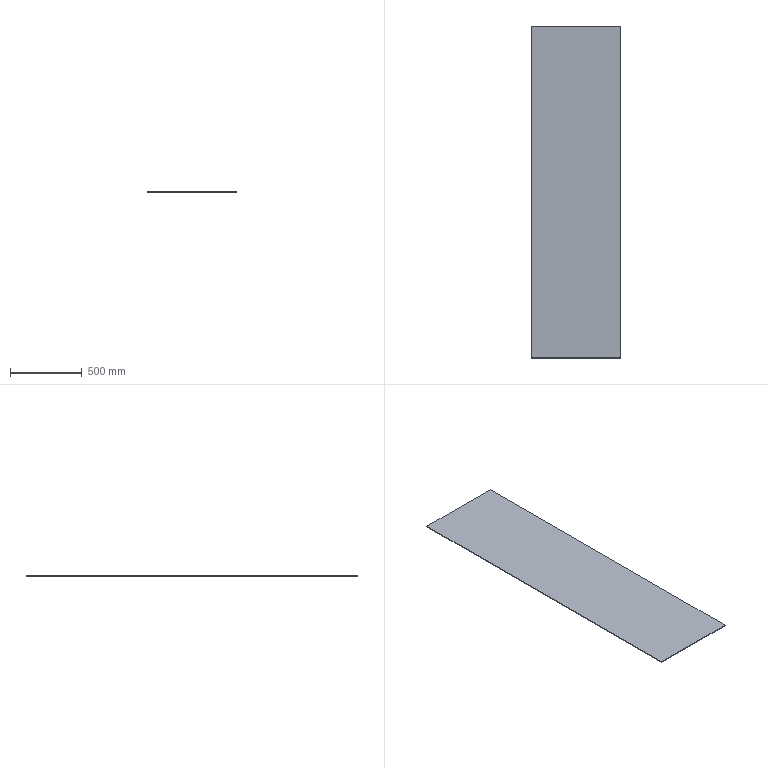Part | SolidWorks | features Extrusion 1, HoleWzd 1 | 1 solid | 6 faces | box 624 x 2310 x 5 mm | volume 7207200 mm3 | plane 6
STEP:
#1=CARTESIAN_POINT('',(312.,-1155.,0.));
#2=VERTEX_POINT('',#1);
#3=CARTESIAN_POINT('',(312.,1155.,0.));
#4=VERTEX_POINT('',#3);
#5=CARTESIAN_POINT('',(312.,1155.,0.));
#6=DIRECTION('',(0.,1.,0.));
#7=VECTOR('',#6,1000.);
#8=LINE('',#5,#7);
#9=EDGE_CURVE('',#2,#4,#8,.T.);
#10=ORIENTED_EDGE('',*,*,#9,.T.);
#11=CARTESIAN_POINT('',(312.,1155.,5.));
#12=VERTEX_POINT('',#11);
#13=CARTESIAN_POINT('',(312.,1155.,5.));
#14=DIRECTION('',(0.,0.,-1.));
#15=VECTOR('',#14,1000.);
#16=LINE('',#13,#15);
#17=EDGE_CURVE('',#12,#4,#16,.T.);
#18=ORIENTED_EDGE('',*,*,#17,.F.);
#19=CARTESIAN_POINT('',(312.,-1155.,5.));
#20=VERTEX_POINT('',#19);
#21=CARTESIAN_POINT('',(312.,1155.,5.));
#22=DIRECTION('',(0.,1.,0.));
#23=VECTOR('',#22,1000.);
#24=LINE('',#21,#23);
#25=EDGE_CURVE('',#20,#12,#24,.T.);
#26=ORIENTED_EDGE('',*,*,#25,.F.);
#27=CARTESIAN_POINT('',(312.,-1155.,5.));
#28=DIRECTION('',(0.,0.,-1.));
#29=VECTOR('',#28,1000.);
#30=LINE('',#27,#29);
#31=EDGE_CURVE('',#20,#2,#30,.T.);
#32=ORIENTED_EDGE('',*,*,#31,.T.);
#33=EDGE_LOOP('',(#10,#18,#26,#32));
#34=FACE_OUTER_BOUND('',#33,.T.);
#35=CARTESIAN_POINT('',(312.,1155.,5.));
#36=DIRECTION('',(-1.,0.,0.));
#37=DIRECTION('',(0.,-1.,0.));
#38=AXIS2_PLACEMENT_3D('',#35,#36,#37);
#39=PLANE('',#38);
#40=ADVANCED_FACE('',(#34),#39,.F.);
#41=CARTESIAN_POINT('',(-312.,1155.,0.));
#42=VERTEX_POINT('',#41);
#43=CARTESIAN_POINT('',(-312.,1155.,0.));
#44=DIRECTION('',(-1.,0.,0.));
#45=VECTOR('',#44,1000.);
#46=LINE('',#43,#45);
#47=EDGE_CURVE('',#4,#42,#46,.T.);
#48=ORIENTED_EDGE('',*,*,#47,.T.);
#49=CARTESIAN_POINT('',(-312.,1155.,5.));
#50=VERTEX_POINT('',#49);
#51=CARTESIAN_POINT('',(-312.,1155.,5.));
#52=DIRECTION('',(0.,0.,-1.));
#53=VECTOR('',#52,1000.);
#54=LINE('',#51,#53);
#55=EDGE_CURVE('',#50,#42,#54,.T.);
#56=ORIENTED_EDGE('',*,*,#55,.F.);
#57=CARTESIAN_POINT('',(-312.,1155.,5.));
#58=DIRECTION('',(-1.,0.,0.));
#59=VECTOR('',#58,1000.);
#60=LINE('',#57,#59);
#61=EDGE_CURVE('',#12,#50,#60,.T.);
#62=ORIENTED_EDGE('',*,*,#61,.F.);
#63=ORIENTED_EDGE('',*,*,#17,.T.);
#64=EDGE_LOOP('',(#48,#56,#62,#63));
#65=FACE_OUTER_BOUND('',#64,.T.);
#66=CARTESIAN_POINT('',(-312.,1155.,5.));
#67=DIRECTION('',(0.,-1.,0.));
#68=DIRECTION('',(0.,0.,-1.));
#69=AXIS2_PLACEMENT_3D('',#66,#67,#68);
#70=PLANE('',#69);
#71=ADVANCED_FACE('',(#65),#70,.F.);
#72=CARTESIAN_POINT('',(-312.,-1155.,0.));
#73=VERTEX_POINT('',#72);
#74=CARTESIAN_POINT('',(-312.,1155.,0.));
#75=DIRECTION('',(0.,-1.,0.));
#76=VECTOR('',#75,1000.);
#77=LINE('',#74,#76);
#78=EDGE_CURVE('',#42,#73,#77,.T.);
#79=ORIENTED_EDGE('',*,*,#78,.T.);
#80=CARTESIAN_POINT('',(-312.,-1155.,5.));
#81=VERTEX_POINT('',#80);
#82=CARTESIAN_POINT('',(-312.,-1155.,5.));
#83=DIRECTION('',(0.,0.,-1.));
#84=VECTOR('',#83,1000.);
#85=LINE('',#82,#84);
#86=EDGE_CURVE('',#81,#73,#85,.T.);
#87=ORIENTED_EDGE('',*,*,#86,.F.);
#88=CARTESIAN_POINT('',(-312.,1155.,5.));
#89=DIRECTION('',(0.,-1.,0.));
#90=VECTOR('',#89,1000.);
#91=LINE('',#88,#90);
#92=EDGE_CURVE('',#50,#81,#91,.T.);
#93=ORIENTED_EDGE('',*,*,#92,.F.);
#94=ORIENTED_EDGE('',*,*,#55,.T.);
#95=EDGE_LOOP('',(#79,#87,#93,#94));
#96=FACE_OUTER_BOUND('',#95,.T.);
#97=CARTESIAN_POINT('',(-312.,1155.,5.));
#98=DIRECTION('',(1.,0.,0.));
#99=DIRECTION('',(0.,1.,0.));
#100=AXIS2_PLACEMENT_3D('',#97,#98,#99);
#101=PLANE('',#100);
#102=ADVANCED_FACE('',(#96),#101,.F.);
#103=CARTESIAN_POINT('',(-312.,-1155.,0.));
#104=DIRECTION('',(1.,0.,0.));
#105=VECTOR('',#104,1000.);
#106=LINE('',#103,#105);
#107=EDGE_CURVE('',#73,#2,#106,.T.);
#108=ORIENTED_EDGE('',*,*,#107,.T.);
#109=ORIENTED_EDGE('',*,*,#31,.F.);
#110=CARTESIAN_POINT('',(-312.,-1155.,5.));
#111=DIRECTION('',(1.,0.,0.));
#112=VECTOR('',#111,1000.);
#113=LINE('',#110,#112);
#114=EDGE_CURVE('',#81,#20,#113,.T.);
#115=ORIENTED_EDGE('',*,*,#114,.F.);
#116=ORIENTED_EDGE('',*,*,#86,.T.);
#117=EDGE_LOOP('',(#108,#109,#115,#116));
#118=FACE_OUTER_BOUND('',#117,.T.);
#119=CARTESIAN_POINT('',(-312.,-1155.,5.));
#120=DIRECTION('',(0.,1.,0.));
#121=DIRECTION('',(0.,0.,1.));
#122=AXIS2_PLACEMENT_3D('',#119,#120,#121);
#123=PLANE('',#122);
#124=ADVANCED_FACE('',(#118),#123,.F.);
#125=ORIENTED_EDGE('',*,*,#25,.T.);
#126=ORIENTED_EDGE('',*,*,#61,.T.);
#127=ORIENTED_EDGE('',*,*,#92,.T.);
#128=ORIENTED_EDGE('',*,*,#114,.T.);
#129=EDGE_LOOP('',(#125,#126,#127,#128));
#130=FACE_OUTER_BOUND('',#129,.T.);
#131=CARTESIAN_POINT('',(0.,0.,5.));
#132=DIRECTION('',(0.,0.,1.));
#133=DIRECTION('',(1.,0.,0.));
#134=AXIS2_PLACEMENT_3D('',#131,#132,#133);
#135=PLANE('',#134);
#136=ADVANCED_FACE('',(#130),#135,.T.);
#137=ORIENTED_EDGE('',*,*,#9,.F.);
#138=ORIENTED_EDGE('',*,*,#107,.F.);
#139=ORIENTED_EDGE('',*,*,#78,.F.);
#140=ORIENTED_EDGE('',*,*,#47,.F.);
#141=EDGE_LOOP('',(#137,#138,#139,#140));
#142=FACE_OUTER_BOUND('',#141,.T.);
#143=CARTESIAN_POINT('',(0.,0.,0.));
#144=DIRECTION('',(0.,0.,1.));
#145=DIRECTION('',(1.,0.,0.));
#146=AXIS2_PLACEMENT_3D('',#143,#144,#145);
#147=PLANE('',#146);
#148=ADVANCED_FACE('',(#142),#147,.F.);
#149=CLOSED_SHELL('',(#40,#71,#102,#124,#136,#148));
#150=MANIFOLD_SOLID_BREP('',#149);
#151=CARTESIAN_POINT('',(0.,0.,0.));
#152=DIRECTION('',(0.,0.,1.));
#153=DIRECTION('',(1.,0.,0.));
#154=AXIS2_PLACEMENT_3D('',#151,#152,#153);
#155=(LENGTH_UNIT()NAMED_UNIT(*)SI_UNIT(.MILLI.,.METRE.));
#156=UNCERTAINTY_MEASURE_WITH_UNIT(LENGTH_MEASURE(0.00001),#155,'','');
#157=(NAMED_UNIT(*)PLANE_ANGLE_UNIT()SI_UNIT($,.RADIAN.));
#158=(NAMED_UNIT(*)SI_UNIT($,.STERADIAN.)SOLID_ANGLE_UNIT());
#159=(GEOMETRIC_REPRESENTATION_CONTEXT(3)GLOBAL_UNCERTAINTY_ASSIGNED_CONTEXT((#156))GLOBAL_UNIT_ASSIGNED_CONTEXT((#155,#157,#158))REPRESENTATION_CONTEXT('',''));
#160=ADVANCED_BREP_SHAPE_REPRESENTATION('',(#150,#154),#159);